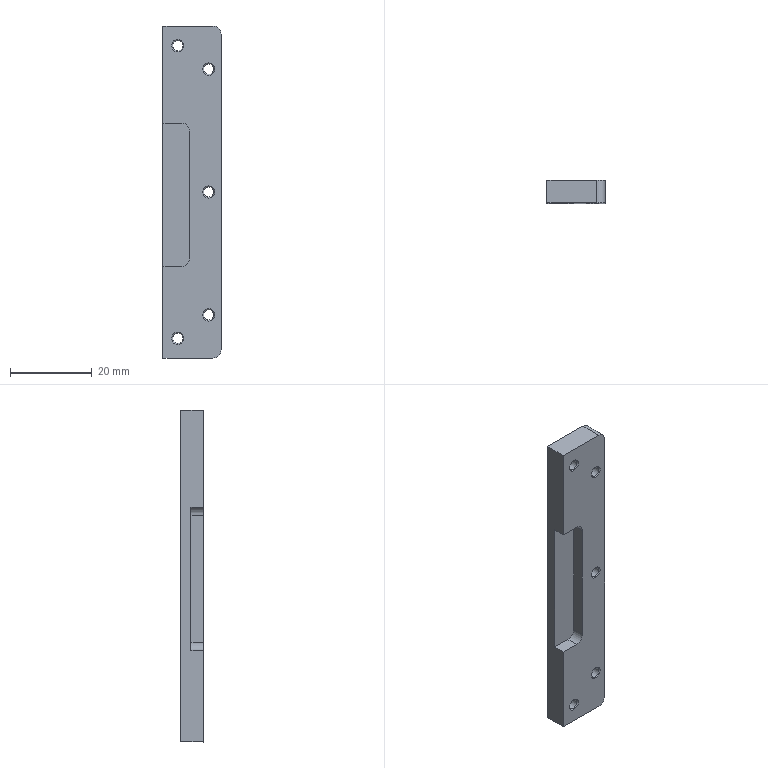Part | STEP file | Screen mounting block 1 | 1 solid | 29 faces | box 14.18 x 5.5 x 81 mm | volume 5488 mm3 | plane 10 | cone 10 | cylinder 9 | commonest cylinder face diameters 2.5 x5 4 x4